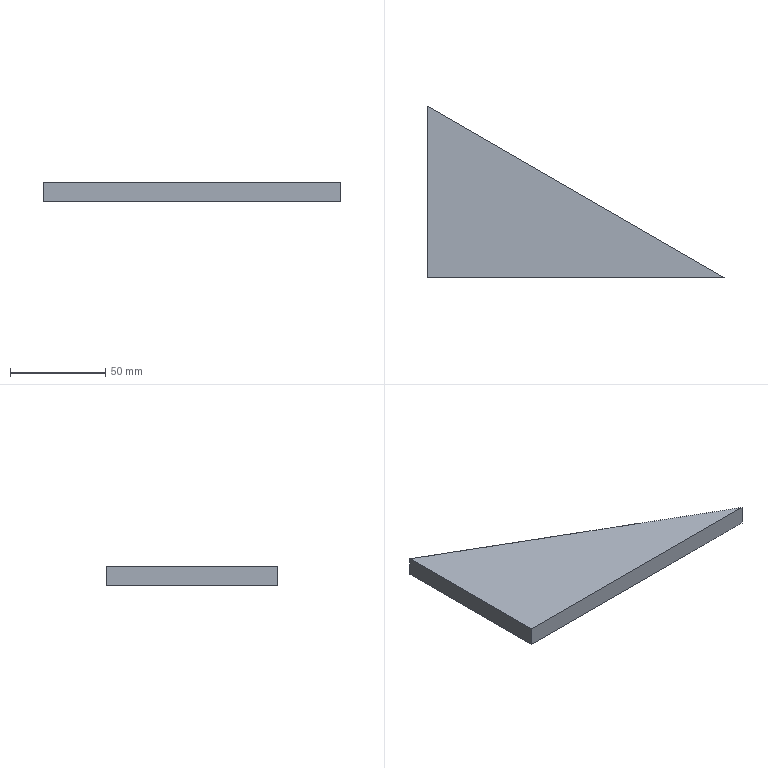Part | SolidWorks | features Extrusion 1 | 1 solid | 5 faces | box 155.885 x 90 x 10 mm | volume 70148 mm3 | plane 5
STEP:
#1=CARTESIAN_POINT('',(155.885,-90.,0.));
#2=VERTEX_POINT('',#1);
#3=CARTESIAN_POINT('',(0.,0.,0.));
#4=VERTEX_POINT('',#3);
#5=CARTESIAN_POINT('',(155.885,-90.,0.));
#6=DIRECTION('',(-0.866,0.5,0.));
#7=VECTOR('',#6,1000.);
#8=LINE('',#5,#7);
#9=EDGE_CURVE('',#2,#4,#8,.T.);
#10=ORIENTED_EDGE('',*,*,#9,.T.);
#11=CARTESIAN_POINT('',(0.,0.,10.));
#12=VERTEX_POINT('',#11);
#13=CARTESIAN_POINT('',(0.,0.,10.));
#14=DIRECTION('',(0.,0.,-1.));
#15=VECTOR('',#14,1000.);
#16=LINE('',#13,#15);
#17=EDGE_CURVE('',#12,#4,#16,.T.);
#18=ORIENTED_EDGE('',*,*,#17,.F.);
#19=CARTESIAN_POINT('',(155.885,-90.,10.));
#20=VERTEX_POINT('',#19);
#21=CARTESIAN_POINT('',(155.885,-90.,10.));
#22=DIRECTION('',(-0.866,0.5,0.));
#23=VECTOR('',#22,1000.);
#24=LINE('',#21,#23);
#25=EDGE_CURVE('',#20,#12,#24,.T.);
#26=ORIENTED_EDGE('',*,*,#25,.F.);
#27=CARTESIAN_POINT('',(155.885,-90.,10.));
#28=DIRECTION('',(0.,0.,-1.));
#29=VECTOR('',#28,1000.);
#30=LINE('',#27,#29);
#31=EDGE_CURVE('',#20,#2,#30,.T.);
#32=ORIENTED_EDGE('',*,*,#31,.T.);
#33=EDGE_LOOP('',(#10,#18,#26,#32));
#34=FACE_OUTER_BOUND('',#33,.T.);
#35=CARTESIAN_POINT('',(155.885,-90.,10.));
#36=DIRECTION('',(-0.5,-0.866,0.));
#37=DIRECTION('',(0.866,-0.5,0.));
#38=AXIS2_PLACEMENT_3D('',#35,#36,#37);
#39=PLANE('',#38);
#40=ADVANCED_FACE('',(#34),#39,.F.);
#41=CARTESIAN_POINT('',(0.,-90.,0.));
#42=VERTEX_POINT('',#41);
#43=CARTESIAN_POINT('',(0.,0.,0.));
#44=DIRECTION('',(0.,-1.,0.));
#45=VECTOR('',#44,1000.);
#46=LINE('',#43,#45);
#47=EDGE_CURVE('',#4,#42,#46,.T.);
#48=ORIENTED_EDGE('',*,*,#47,.T.);
#49=CARTESIAN_POINT('',(0.,-90.,10.));
#50=VERTEX_POINT('',#49);
#51=CARTESIAN_POINT('',(0.,-90.,10.));
#52=DIRECTION('',(0.,0.,-1.));
#53=VECTOR('',#52,1000.);
#54=LINE('',#51,#53);
#55=EDGE_CURVE('',#50,#42,#54,.T.);
#56=ORIENTED_EDGE('',*,*,#55,.F.);
#57=CARTESIAN_POINT('',(0.,0.,10.));
#58=DIRECTION('',(0.,-1.,0.));
#59=VECTOR('',#58,1000.);
#60=LINE('',#57,#59);
#61=EDGE_CURVE('',#12,#50,#60,.T.);
#62=ORIENTED_EDGE('',*,*,#61,.F.);
#63=ORIENTED_EDGE('',*,*,#17,.T.);
#64=EDGE_LOOP('',(#48,#56,#62,#63));
#65=FACE_OUTER_BOUND('',#64,.T.);
#66=CARTESIAN_POINT('',(0.,0.,10.));
#67=DIRECTION('',(1.,0.,0.));
#68=DIRECTION('',(0.,0.,-1.));
#69=AXIS2_PLACEMENT_3D('',#66,#67,#68);
#70=PLANE('',#69);
#71=ADVANCED_FACE('',(#65),#70,.F.);
#72=CARTESIAN_POINT('',(0.,-90.,0.));
#73=DIRECTION('',(1.,0.,0.));
#74=VECTOR('',#73,1000.);
#75=LINE('',#72,#74);
#76=EDGE_CURVE('',#42,#2,#75,.T.);
#77=ORIENTED_EDGE('',*,*,#76,.T.);
#78=ORIENTED_EDGE('',*,*,#31,.F.);
#79=CARTESIAN_POINT('',(0.,-90.,10.));
#80=DIRECTION('',(1.,0.,0.));
#81=VECTOR('',#80,1000.);
#82=LINE('',#79,#81);
#83=EDGE_CURVE('',#50,#20,#82,.T.);
#84=ORIENTED_EDGE('',*,*,#83,.F.);
#85=ORIENTED_EDGE('',*,*,#55,.T.);
#86=EDGE_LOOP('',(#77,#78,#84,#85));
#87=FACE_OUTER_BOUND('',#86,.T.);
#88=CARTESIAN_POINT('',(0.,-90.,10.));
#89=DIRECTION('',(0.,1.,0.));
#90=DIRECTION('',(0.,0.,1.));
#91=AXIS2_PLACEMENT_3D('',#88,#89,#90);
#92=PLANE('',#91);
#93=ADVANCED_FACE('',(#87),#92,.F.);
#94=ORIENTED_EDGE('',*,*,#25,.T.);
#95=ORIENTED_EDGE('',*,*,#61,.T.);
#96=ORIENTED_EDGE('',*,*,#83,.T.);
#97=EDGE_LOOP('',(#94,#95,#96));
#98=FACE_OUTER_BOUND('',#97,.T.);
#99=CARTESIAN_POINT('',(0.,0.,10.));
#100=DIRECTION('',(0.,0.,1.));
#101=DIRECTION('',(1.,0.,0.));
#102=AXIS2_PLACEMENT_3D('',#99,#100,#101);
#103=PLANE('',#102);
#104=ADVANCED_FACE('',(#98),#103,.T.);
#105=ORIENTED_EDGE('',*,*,#9,.F.);
#106=ORIENTED_EDGE('',*,*,#76,.F.);
#107=ORIENTED_EDGE('',*,*,#47,.F.);
#108=EDGE_LOOP('',(#105,#106,#107));
#109=FACE_OUTER_BOUND('',#108,.T.);
#110=CARTESIAN_POINT('',(0.,0.,0.));
#111=DIRECTION('',(0.,0.,1.));
#112=DIRECTION('',(1.,0.,0.));
#113=AXIS2_PLACEMENT_3D('',#110,#111,#112);
#114=PLANE('',#113);
#115=ADVANCED_FACE('',(#109),#114,.F.);
#116=CLOSED_SHELL('',(#40,#71,#93,#104,#115));
#117=MANIFOLD_SOLID_BREP('',#116);
#118=CARTESIAN_POINT('',(0.,0.,0.));
#119=DIRECTION('',(0.,0.,1.));
#120=DIRECTION('',(1.,0.,0.));
#121=AXIS2_PLACEMENT_3D('',#118,#119,#120);
#122=(LENGTH_UNIT()NAMED_UNIT(*)SI_UNIT(.MILLI.,.METRE.));
#123=UNCERTAINTY_MEASURE_WITH_UNIT(LENGTH_MEASURE(0.00001),#122,'','');
#124=(NAMED_UNIT(*)PLANE_ANGLE_UNIT()SI_UNIT($,.RADIAN.));
#125=(NAMED_UNIT(*)SI_UNIT($,.STERADIAN.)SOLID_ANGLE_UNIT());
#126=(GEOMETRIC_REPRESENTATION_CONTEXT(3)GLOBAL_UNCERTAINTY_ASSIGNED_CONTEXT((#123))GLOBAL_UNIT_ASSIGNED_CONTEXT((#122,#124,#125))REPRESENTATION_CONTEXT('',''));
#127=ADVANCED_BREP_SHAPE_REPRESENTATION('',(#117,#121),#126);